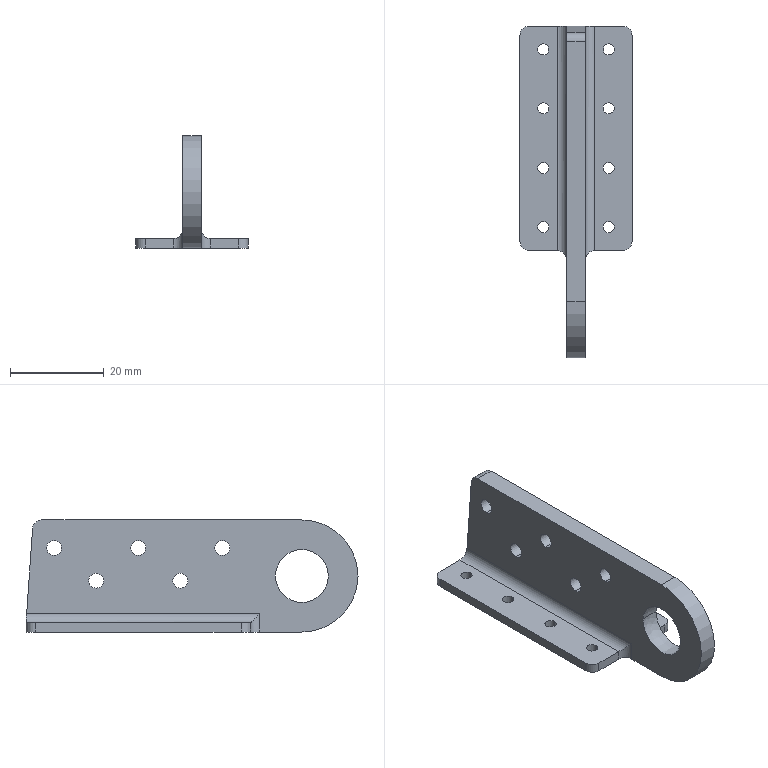Part | SolidWorks | features BaseBody 1 | 1 solid | 51 faces | box 24 x 71 x 24 mm | volume 7830 mm3 | cylinder 36 | plane 13 | spline 2 | commonest cylinder face diameters 2.4 x16 3.2 x10 4 x9 24 x1